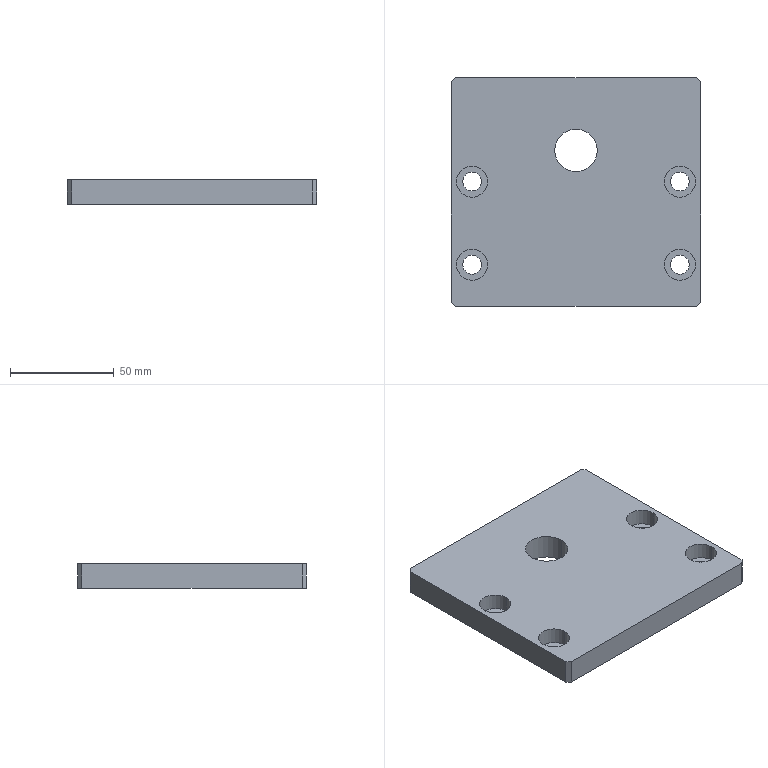Part | SolidWorks | features BaseBody 1 | 1 solid | 32 faces | box 120 x 110 x 12 mm | volume 147670 mm3 | cylinder 18 | plane 14 | commonest cylinder face diameters 9 x8 15 x8 20.5 x2
STEP:
#1=CARTESIAN_POINT('',(54.5,5.,0.));
#2=VERTEX_POINT('',#1);
#3=CARTESIAN_POINT('',(45.5,5.,0.));
#4=VERTEX_POINT('',#3);
#5=CARTESIAN_POINT('',(50.,5.,0.));
#6=DIRECTION('',(0.,0.,-1.));
#7=DIRECTION('',(1.,0.,0.));
#8=AXIS2_PLACEMENT_3D('',#5,#6,#7);
#9=CIRCLE('',#8,4.5);
#10=EDGE_CURVE('',#2,#4,#9,.T.);
#11=ORIENTED_EDGE('',*,*,#10,.T.);
#12=CARTESIAN_POINT('',(45.5,5.,4.));
#13=VERTEX_POINT('',#12);
#14=CARTESIAN_POINT('',(45.5,5.,12.));
#15=DIRECTION('',(0.,0.,1.));
#16=VECTOR('',#15,1000.);
#17=LINE('',#14,#16);
#18=EDGE_CURVE('',#4,#13,#17,.T.);
#19=ORIENTED_EDGE('',*,*,#18,.T.);
#20=CARTESIAN_POINT('',(54.5,5.,4.));
#21=VERTEX_POINT('',#20);
#22=CARTESIAN_POINT('',(50.,5.,4.));
#23=DIRECTION('',(0.,0.,-1.));
#24=DIRECTION('',(1.,0.,0.));
#25=AXIS2_PLACEMENT_3D('',#22,#23,#24);
#26=CIRCLE('',#25,4.5);
#27=EDGE_CURVE('',#21,#13,#26,.T.);
#28=ORIENTED_EDGE('',*,*,#27,.F.);
#29=CARTESIAN_POINT('',(54.5,5.,12.));
#30=DIRECTION('',(0.,0.,1.));
#31=VECTOR('',#30,1000.);
#32=LINE('',#29,#31);
#33=EDGE_CURVE('',#2,#21,#32,.T.);
#34=ORIENTED_EDGE('',*,*,#33,.F.);
#35=EDGE_LOOP('',(#11,#19,#28,#34));
#36=FACE_OUTER_BOUND('',#35,.T.);
#37=CARTESIAN_POINT('',(50.,5.,12.));
#38=DIRECTION('',(0.,0.,1.));
#39=DIRECTION('',(1.,0.,0.));
#40=AXIS2_PLACEMENT_3D('',#37,#38,#39);
#41=CYLINDRICAL_SURFACE('',#40,4.5);
#42=ADVANCED_FACE('',(#36),#41,.F.);
#43=CARTESIAN_POINT('',(54.5,-35.,0.));
#44=VERTEX_POINT('',#43);
#45=CARTESIAN_POINT('',(45.5,-35.,0.));
#46=VERTEX_POINT('',#45);
#47=CARTESIAN_POINT('',(50.,-35.,0.));
#48=DIRECTION('',(0.,0.,-1.));
#49=DIRECTION('',(1.,0.,0.));
#50=AXIS2_PLACEMENT_3D('',#47,#48,#49);
#51=CIRCLE('',#50,4.5);
#52=EDGE_CURVE('',#44,#46,#51,.T.);
#53=ORIENTED_EDGE('',*,*,#52,.T.);
#54=CARTESIAN_POINT('',(45.5,-35.,4.));
#55=VERTEX_POINT('',#54);
#56=CARTESIAN_POINT('',(45.5,-35.,12.));
#57=DIRECTION('',(0.,0.,1.));
#58=VECTOR('',#57,1000.);
#59=LINE('',#56,#58);
#60=EDGE_CURVE('',#46,#55,#59,.T.);
#61=ORIENTED_EDGE('',*,*,#60,.T.);
#62=CARTESIAN_POINT('',(54.5,-35.,4.));
#63=VERTEX_POINT('',#62);
#64=CARTESIAN_POINT('',(50.,-35.,4.));
#65=DIRECTION('',(0.,0.,-1.));
#66=DIRECTION('',(1.,0.,0.));
#67=AXIS2_PLACEMENT_3D('',#64,#65,#66);
#68=CIRCLE('',#67,4.5);
#69=EDGE_CURVE('',#63,#55,#68,.T.);
#70=ORIENTED_EDGE('',*,*,#69,.F.);
#71=CARTESIAN_POINT('',(54.5,-35.,12.));
#72=DIRECTION('',(0.,0.,1.));
#73=VECTOR('',#72,1000.);
#74=LINE('',#71,#73);
#75=EDGE_CURVE('',#44,#63,#74,.T.);
#76=ORIENTED_EDGE('',*,*,#75,.F.);
#77=EDGE_LOOP('',(#53,#61,#70,#76));
#78=FACE_OUTER_BOUND('',#77,.T.);
#79=CARTESIAN_POINT('',(50.,-35.,12.));
#80=DIRECTION('',(0.,0.,1.));
#81=DIRECTION('',(1.,0.,0.));
#82=AXIS2_PLACEMENT_3D('',#79,#80,#81);
#83=CYLINDRICAL_SURFACE('',#82,4.5);
#84=ADVANCED_FACE('',(#78),#83,.F.);
#85=CARTESIAN_POINT('',(-45.5,-35.,0.));
#86=VERTEX_POINT('',#85);
#87=CARTESIAN_POINT('',(-54.5,-35.,0.));
#88=VERTEX_POINT('',#87);
#89=CARTESIAN_POINT('',(-50.,-35.,0.));
#90=DIRECTION('',(0.,0.,-1.));
#91=DIRECTION('',(1.,0.,0.));
#92=AXIS2_PLACEMENT_3D('',#89,#90,#91);
#93=CIRCLE('',#92,4.5);
#94=EDGE_CURVE('',#86,#88,#93,.T.);
#95=ORIENTED_EDGE('',*,*,#94,.T.);
#96=CARTESIAN_POINT('',(-54.5,-35.,4.));
#97=VERTEX_POINT('',#96);
#98=CARTESIAN_POINT('',(-54.5,-35.,12.));
#99=DIRECTION('',(0.,0.,1.));
#100=VECTOR('',#99,1000.);
#101=LINE('',#98,#100);
#102=EDGE_CURVE('',#88,#97,#101,.T.);
#103=ORIENTED_EDGE('',*,*,#102,.T.);
#104=CARTESIAN_POINT('',(-45.5,-35.,4.));
#105=VERTEX_POINT('',#104);
#106=CARTESIAN_POINT('',(-50.,-35.,4.));
#107=DIRECTION('',(0.,0.,-1.));
#108=DIRECTION('',(1.,0.,0.));
#109=AXIS2_PLACEMENT_3D('',#106,#107,#108);
#110=CIRCLE('',#109,4.5);
#111=EDGE_CURVE('',#105,#97,#110,.T.);
#112=ORIENTED_EDGE('',*,*,#111,.F.);
#113=CARTESIAN_POINT('',(-45.5,-35.,12.));
#114=DIRECTION('',(0.,0.,1.));
#115=VECTOR('',#114,1000.);
#116=LINE('',#113,#115);
#117=EDGE_CURVE('',#86,#105,#116,.T.);
#118=ORIENTED_EDGE('',*,*,#117,.F.);
#119=EDGE_LOOP('',(#95,#103,#112,#118));
#120=FACE_OUTER_BOUND('',#119,.T.);
#121=CARTESIAN_POINT('',(-50.,-35.,12.));
#122=DIRECTION('',(0.,0.,1.));
#123=DIRECTION('',(1.,0.,0.));
#124=AXIS2_PLACEMENT_3D('',#121,#122,#123);
#125=CYLINDRICAL_SURFACE('',#124,4.5);
#126=ADVANCED_FACE('',(#120),#125,.F.);
#127=CARTESIAN_POINT('',(-45.5,5.,0.));
#128=VERTEX_POINT('',#127);
#129=CARTESIAN_POINT('',(-54.5,5.,0.));
#130=VERTEX_POINT('',#129);
#131=CARTESIAN_POINT('',(-50.,5.,0.));
#132=DIRECTION('',(0.,0.,-1.));
#133=DIRECTION('',(1.,0.,0.));
#134=AXIS2_PLACEMENT_3D('',#131,#132,#133);
#135=CIRCLE('',#134,4.5);
#136=EDGE_CURVE('',#128,#130,#135,.T.);
#137=ORIENTED_EDGE('',*,*,#136,.T.);
#138=CARTESIAN_POINT('',(-54.5,5.,4.));
#139=VERTEX_POINT('',#138);
#140=CARTESIAN_POINT('',(-54.5,5.,12.));
#141=DIRECTION('',(0.,0.,1.));
#142=VECTOR('',#141,1000.);
#143=LINE('',#140,#142);
#144=EDGE_CURVE('',#130,#139,#143,.T.);
#145=ORIENTED_EDGE('',*,*,#144,.T.);
#146=CARTESIAN_POINT('',(-45.5,5.,4.));
#147=VERTEX_POINT('',#146);
#148=CARTESIAN_POINT('',(-50.,5.,4.));
#149=DIRECTION('',(0.,0.,-1.));
#150=DIRECTION('',(1.,0.,0.));
#151=AXIS2_PLACEMENT_3D('',#148,#149,#150);
#152=CIRCLE('',#151,4.5);
#153=EDGE_CURVE('',#147,#139,#152,.T.);
#154=ORIENTED_EDGE('',*,*,#153,.F.);
#155=CARTESIAN_POINT('',(-45.5,5.,12.));
#156=DIRECTION('',(0.,0.,1.));
#157=VECTOR('',#156,1000.);
#158=LINE('',#155,#157);
#159=EDGE_CURVE('',#128,#147,#158,.T.);
#160=ORIENTED_EDGE('',*,*,#159,.F.);
#161=EDGE_LOOP('',(#137,#145,#154,#160));
#162=FACE_OUTER_BOUND('',#161,.T.);
#163=CARTESIAN_POINT('',(-50.,5.,12.));
#164=DIRECTION('',(0.,0.,1.));
#165=DIRECTION('',(1.,0.,0.));
#166=AXIS2_PLACEMENT_3D('',#163,#164,#165);
#167=CYLINDRICAL_SURFACE('',#166,4.5);
#168=ADVANCED_FACE('',(#162),#167,.F.);
#169=CARTESIAN_POINT('',(10.25,20.,0.));
#170=VERTEX_POINT('',#169);
#171=CARTESIAN_POINT('',(-10.25,20.,0.));
#172=VERTEX_POINT('',#171);
#173=CARTESIAN_POINT('',(0.,20.,0.));
#174=DIRECTION('',(0.,0.,-1.));
#175=DIRECTION('',(1.,0.,0.));
#176=AXIS2_PLACEMENT_3D('',#173,#174,#175);
#177=CIRCLE('',#176,10.25);
#178=EDGE_CURVE('',#170,#172,#177,.T.);
#179=ORIENTED_EDGE('',*,*,#178,.T.);
#180=CARTESIAN_POINT('',(-10.25,20.,12.));
#181=VERTEX_POINT('',#180);
#182=CARTESIAN_POINT('',(-10.25,20.,12.));
#183=DIRECTION('',(0.,0.,1.));
#184=VECTOR('',#183,1000.);
#185=LINE('',#182,#184);
#186=EDGE_CURVE('',#172,#181,#185,.T.);
#187=ORIENTED_EDGE('',*,*,#186,.T.);
#188=CARTESIAN_POINT('',(10.25,20.,12.));
#189=VERTEX_POINT('',#188);
#190=CARTESIAN_POINT('',(0.,20.,12.));
#191=DIRECTION('',(0.,0.,-1.));
#192=DIRECTION('',(1.,0.,0.));
#193=AXIS2_PLACEMENT_3D('',#190,#191,#192);
#194=CIRCLE('',#193,10.25);
#195=EDGE_CURVE('',#189,#181,#194,.T.);
#196=ORIENTED_EDGE('',*,*,#195,.F.);
#197=CARTESIAN_POINT('',(10.25,20.,12.));
#198=DIRECTION('',(0.,0.,1.));
#199=VECTOR('',#198,1000.);
#200=LINE('',#197,#199);
#201=EDGE_CURVE('',#170,#189,#200,.T.);
#202=ORIENTED_EDGE('',*,*,#201,.F.);
#203=EDGE_LOOP('',(#179,#187,#196,#202));
#204=FACE_OUTER_BOUND('',#203,.T.);
#205=CARTESIAN_POINT('',(0.,20.,12.));
#206=DIRECTION('',(0.,0.,1.));
#207=DIRECTION('',(1.,0.,0.));
#208=AXIS2_PLACEMENT_3D('',#205,#206,#207);
#209=CYLINDRICAL_SURFACE('',#208,10.25);
#210=ADVANCED_FACE('',(#204),#209,.F.);
#211=CARTESIAN_POINT('',(57.5,5.,4.));
#212=VERTEX_POINT('',#211);
#213=CARTESIAN_POINT('',(42.5,5.,4.));
#214=VERTEX_POINT('',#213);
#215=CARTESIAN_POINT('',(50.,5.,4.));
#216=DIRECTION('',(0.,0.,-1.));
#217=DIRECTION('',(1.,0.,0.));
#218=AXIS2_PLACEMENT_3D('',#215,#216,#217);
#219=CIRCLE('',#218,7.5);
#220=EDGE_CURVE('',#212,#214,#219,.T.);
#221=ORIENTED_EDGE('',*,*,#220,.T.);
#222=CARTESIAN_POINT('',(42.5,5.,12.));
#223=VERTEX_POINT('',#222);
#224=CARTESIAN_POINT('',(42.5,5.,12.));
#225=DIRECTION('',(0.,0.,1.));
#226=VECTOR('',#225,1000.);
#227=LINE('',#224,#226);
#228=EDGE_CURVE('',#214,#223,#227,.T.);
#229=ORIENTED_EDGE('',*,*,#228,.T.);
#230=CARTESIAN_POINT('',(57.5,5.,12.));
#231=VERTEX_POINT('',#230);
#232=CARTESIAN_POINT('',(50.,5.,12.));
#233=DIRECTION('',(0.,0.,-1.));
#234=DIRECTION('',(1.,0.,0.));
#235=AXIS2_PLACEMENT_3D('',#232,#233,#234);
#236=CIRCLE('',#235,7.5);
#237=EDGE_CURVE('',#231,#223,#236,.T.);
#238=ORIENTED_EDGE('',*,*,#237,.F.);
#239=CARTESIAN_POINT('',(57.5,5.,12.));
#240=DIRECTION('',(0.,0.,1.));
#241=VECTOR('',#240,1000.);
#242=LINE('',#239,#241);
#243=EDGE_CURVE('',#212,#231,#242,.T.);
#244=ORIENTED_EDGE('',*,*,#243,.F.);
#245=EDGE_LOOP('',(#221,#229,#238,#244));
#246=FACE_OUTER_BOUND('',#245,.T.);
#247=CARTESIAN_POINT('',(50.,5.,12.));
#248=DIRECTION('',(0.,0.,1.));
#249=DIRECTION('',(1.,0.,0.));
#250=AXIS2_PLACEMENT_3D('',#247,#248,#249);
#251=CYLINDRICAL_SURFACE('',#250,7.5);
#252=ADVANCED_FACE('',(#246),#251,.F.);
#253=CARTESIAN_POINT('',(57.5,-35.,4.));
#254=VERTEX_POINT('',#253);
#255=CARTESIAN_POINT('',(42.5,-35.,4.));
#256=VERTEX_POINT('',#255);
#257=CARTESIAN_POINT('',(50.,-35.,4.));
#258=DIRECTION('',(0.,0.,-1.));
#259=DIRECTION('',(1.,0.,0.));
#260=AXIS2_PLACEMENT_3D('',#257,#258,#259);
#261=CIRCLE('',#260,7.5);
#262=EDGE_CURVE('',#254,#256,#261,.T.);
#263=ORIENTED_EDGE('',*,*,#262,.T.);
#264=CARTESIAN_POINT('',(42.5,-35.,12.));
#265=VERTEX_POINT('',#264);
#266=CARTESIAN_POINT('',(42.5,-35.,12.));
#267=DIRECTION('',(0.,0.,1.));
#268=VECTOR('',#267,1000.);
#269=LINE('',#266,#268);
#270=EDGE_CURVE('',#256,#265,#269,.T.);
#271=ORIENTED_EDGE('',*,*,#270,.T.);
#272=CARTESIAN_POINT('',(57.5,-35.,12.));
#273=VERTEX_POINT('',#272);
#274=CARTESIAN_POINT('',(50.,-35.,12.));
#275=DIRECTION('',(0.,0.,-1.));
#276=DIRECTION('',(1.,0.,0.));
#277=AXIS2_PLACEMENT_3D('',#274,#275,#276);
#278=CIRCLE('',#277,7.5);
#279=EDGE_CURVE('',#273,#265,#278,.T.);
#280=ORIENTED_EDGE('',*,*,#279,.F.);
#281=CARTESIAN_POINT('',(57.5,-35.,12.));
#282=DIRECTION('',(0.,0.,1.));
#283=VECTOR('',#282,1000.);
#284=LINE('',#281,#283);
#285=EDGE_CURVE('',#254,#273,#284,.T.);
#286=ORIENTED_EDGE('',*,*,#285,.F.);
#287=EDGE_LOOP('',(#263,#271,#280,#286));
#288=FACE_OUTER_BOUND('',#287,.T.);
#289=CARTESIAN_POINT('',(50.,-35.,12.));
#290=DIRECTION('',(0.,0.,1.));
#291=DIRECTION('',(1.,0.,0.));
#292=AXIS2_PLACEMENT_3D('',#289,#290,#291);
#293=CYLINDRICAL_SURFACE('',#292,7.5);
#294=ADVANCED_FACE('',(#288),#293,.F.);
#295=CARTESIAN_POINT('',(-42.5,-35.,4.));
#296=VERTEX_POINT('',#295);
#297=CARTESIAN_POINT('',(-57.5,-35.,4.));
#298=VERTEX_POINT('',#297);
#299=CARTESIAN_POINT('',(-50.,-35.,4.));
#300=DIRECTION('',(0.,0.,-1.));
#301=DIRECTION('',(1.,0.,0.));
#302=AXIS2_PLACEMENT_3D('',#299,#300,#301);
#303=CIRCLE('',#302,7.5);
#304=EDGE_CURVE('',#296,#298,#303,.T.);
#305=ORIENTED_EDGE('',*,*,#304,.T.);
#306=CARTESIAN_POINT('',(-57.5,-35.,12.));
#307=VERTEX_POINT('',#306);
#308=CARTESIAN_POINT('',(-57.5,-35.,12.));
#309=DIRECTION('',(0.,0.,1.));
#310=VECTOR('',#309,1000.);
#311=LINE('',#308,#310);
#312=EDGE_CURVE('',#298,#307,#311,.T.);
#313=ORIENTED_EDGE('',*,*,#312,.T.);
#314=CARTESIAN_POINT('',(-42.5,-35.,12.));
#315=VERTEX_POINT('',#314);
#316=CARTESIAN_POINT('',(-50.,-35.,12.));
#317=DIRECTION('',(0.,0.,-1.));
#318=DIRECTION('',(1.,0.,0.));
#319=AXIS2_PLACEMENT_3D('',#316,#317,#318);
#320=CIRCLE('',#319,7.5);
#321=EDGE_CURVE('',#315,#307,#320,.T.);
#322=ORIENTED_EDGE('',*,*,#321,.F.);
#323=CARTESIAN_POINT('',(-42.5,-35.,12.));
#324=DIRECTION('',(0.,0.,1.));
#325=VECTOR('',#324,1000.);
#326=LINE('',#323,#325);
#327=EDGE_CURVE('',#296,#315,#326,.T.);
#328=ORIENTED_EDGE('',*,*,#327,.F.);
#329=EDGE_LOOP('',(#305,#313,#322,#328));
#330=FACE_OUTER_BOUND('',#329,.T.);
#331=CARTESIAN_POINT('',(-50.,-35.,12.));
#332=DIRECTION('',(0.,0.,1.));
#333=DIRECTION('',(1.,0.,0.));
#334=AXIS2_PLACEMENT_3D('',#331,#332,#333);
#335=CYLINDRICAL_SURFACE('',#334,7.5);
#336=ADVANCED_FACE('',(#330),#335,.F.);
#337=CARTESIAN_POINT('',(-42.5,5.,4.));
#338=VERTEX_POINT('',#337);
#339=CARTESIAN_POINT('',(-57.5,5.,4.));
#340=VERTEX_POINT('',#339);
#341=CARTESIAN_POINT('',(-50.,5.,4.));
#342=DIRECTION('',(0.,0.,-1.));
#343=DIRECTION('',(1.,0.,0.));
#344=AXIS2_PLACEMENT_3D('',#341,#342,#343);
#345=CIRCLE('',#344,7.5);
#346=EDGE_CURVE('',#338,#340,#345,.T.);
#347=ORIENTED_EDGE('',*,*,#346,.T.);
#348=CARTESIAN_POINT('',(-57.5,5.,12.));
#349=VERTEX_POINT('',#348);
#350=CARTESIAN_POINT('',(-57.5,5.,12.));
#351=DIRECTION('',(0.,0.,1.));
#352=VECTOR('',#351,1000.);
#353=LINE('',#350,#352);
#354=EDGE_CURVE('',#340,#349,#353,.T.);
#355=ORIENTED_EDGE('',*,*,#354,.T.);
#356=CARTESIAN_POINT('',(-42.5,5.,12.));
#357=VERTEX_POINT('',#356);
#358=CARTESIAN_POINT('',(-50.,5.,12.));
#359=DIRECTION('',(0.,0.,-1.));
#360=DIRECTION('',(1.,0.,0.));
#361=AXIS2_PLACEMENT_3D('',#358,#359,#360);
#362=CIRCLE('',#361,7.5);
#363=EDGE_CURVE('',#357,#349,#362,.T.);
#364=ORIENTED_EDGE('',*,*,#363,.F.);
#365=CARTESIAN_POINT('',(-42.5,5.,12.));
#366=DIRECTION('',(0.,0.,1.));
#367=VECTOR('',#366,1000.);
#368=LINE('',#365,#367);
#369=EDGE_CURVE('',#338,#357,#368,.T.);
#370=ORIENTED_EDGE('',*,*,#369,.F.);
#371=EDGE_LOOP('',(#347,#355,#364,#370));
#372=FACE_OUTER_BOUND('',#371,.T.);
#373=CARTESIAN_POINT('',(-50.,5.,12.));
#374=DIRECTION('',(0.,0.,1.));
#375=DIRECTION('',(1.,0.,0.));
#376=AXIS2_PLACEMENT_3D('',#373,#374,#375);
#377=CYLINDRICAL_SURFACE('',#376,7.5);
#378=ADVANCED_FACE('',(#372),#377,.F.);
#379=CARTESIAN_POINT('',(-58.,55.,0.));
#380=VERTEX_POINT('',#379);
#381=CARTESIAN_POINT('',(-60.,53.,0.));
#382=VERTEX_POINT('',#381);
#383=CARTESIAN_POINT('',(-58.,55.,0.));
#384=DIRECTION('',(-0.7071,-0.7071,0.));
#385=VECTOR('',#384,1000.);
#386=LINE('',#383,#385);
#387=EDGE_CURVE('',#380,#382,#386,.T.);
#388=ORIENTED_EDGE('',*,*,#387,.F.);
#389=CARTESIAN_POINT('',(58.,55.,0.));
#390=VERTEX_POINT('',#389);
#391=CARTESIAN_POINT('',(0.,55.,0.));
#392=DIRECTION('',(-1.,0.,0.));
#393=VECTOR('',#392,1000.);
#394=LINE('',#391,#393);
#395=EDGE_CURVE('',#390,#380,#394,.T.);
#396=ORIENTED_EDGE('',*,*,#395,.F.);
#397=CARTESIAN_POINT('',(60.,53.,0.));
#398=VERTEX_POINT('',#397);
#399=CARTESIAN_POINT('',(60.,53.,0.));
#400=DIRECTION('',(-0.7071,0.7071,0.));
#401=VECTOR('',#400,1000.);
#402=LINE('',#399,#401);
#403=EDGE_CURVE('',#398,#390,#402,.T.);
#404=ORIENTED_EDGE('',*,*,#403,.F.);
#405=CARTESIAN_POINT('',(60.,-53.,0.));
#406=VERTEX_POINT('',#405);
#407=CARTESIAN_POINT('',(60.,0.,0.));
#408=DIRECTION('',(0.,1.,0.));
#409=VECTOR('',#408,1000.);
#410=LINE('',#407,#409);
#411=EDGE_CURVE('',#406,#398,#410,.T.);
#412=ORIENTED_EDGE('',*,*,#411,.F.);
#413=CARTESIAN_POINT('',(58.,-55.,0.));
#414=VERTEX_POINT('',#413);
#415=CARTESIAN_POINT('',(58.,-55.,0.));
#416=DIRECTION('',(0.7071,0.7071,0.));
#417=VECTOR('',#416,1000.);
#418=LINE('',#415,#417);
#419=EDGE_CURVE('',#414,#406,#418,.T.);
#420=ORIENTED_EDGE('',*,*,#419,.F.);
#421=CARTESIAN_POINT('',(-58.,-55.,0.));
#422=VERTEX_POINT('',#421);
#423=CARTESIAN_POINT('',(0.,-55.,0.));
#424=DIRECTION('',(1.,0.,0.));
#425=VECTOR('',#424,1000.);
#426=LINE('',#423,#425);
#427=EDGE_CURVE('',#422,#414,#426,.T.);
#428=ORIENTED_EDGE('',*,*,#427,.F.);
#429=CARTESIAN_POINT('',(-60.,-53.,0.));
#430=VERTEX_POINT('',#429);
#431=CARTESIAN_POINT('',(-60.,-53.,0.));
#432=DIRECTION('',(0.7071,-0.7071,0.));
#433=VECTOR('',#432,1000.);
#434=LINE('',#431,#433);
#435=EDGE_CURVE('',#430,#422,#434,.T.);
#436=ORIENTED_EDGE('',*,*,#435,.F.);
#437=CARTESIAN_POINT('',(-60.,0.,0.));
#438=DIRECTION('',(0.,-1.,0.));
#439=VECTOR('',#438,1000.);
#440=LINE('',#437,#439);
#441=EDGE_CURVE('',#382,#430,#440,.T.);
#442=ORIENTED_EDGE('',*,*,#441,.F.);
#443=EDGE_LOOP('',(#388,#396,#404,#412,#420,#428,#436,#442));
#444=FACE_OUTER_BOUND('',#443,.T.);
#445=ORIENTED_EDGE('',*,*,#10,.F.);
#446=CARTESIAN_POINT('',(50.,5.,0.));
#447=DIRECTION('',(0.,0.,-1.));
#448=DIRECTION('',(1.,0.,0.));
#449=AXIS2_PLACEMENT_3D('',#446,#447,#448);
#450=CIRCLE('',#449,4.5);
#451=EDGE_CURVE('',#4,#2,#450,.T.);
#452=ORIENTED_EDGE('',*,*,#451,.F.);
#453=EDGE_LOOP('',(#445,#452));
#454=FACE_BOUND('',#453,.T.);
#455=ORIENTED_EDGE('',*,*,#52,.F.);
#456=CARTESIAN_POINT('',(50.,-35.,0.));
#457=DIRECTION('',(0.,0.,-1.));
#458=DIRECTION('',(1.,0.,0.));
#459=AXIS2_PLACEMENT_3D('',#456,#457,#458);
#460=CIRCLE('',#459,4.5);
#461=EDGE_CURVE('',#46,#44,#460,.T.);
#462=ORIENTED_EDGE('',*,*,#461,.F.);
#463=EDGE_LOOP('',(#455,#462));
#464=FACE_BOUND('',#463,.T.);
#465=ORIENTED_EDGE('',*,*,#94,.F.);
#466=CARTESIAN_POINT('',(-50.,-35.,0.));
#467=DIRECTION('',(0.,0.,-1.));
#468=DIRECTION('',(1.,0.,0.));
#469=AXIS2_PLACEMENT_3D('',#466,#467,#468);
#470=CIRCLE('',#469,4.5);
#471=EDGE_CURVE('',#88,#86,#470,.T.);
#472=ORIENTED_EDGE('',*,*,#471,.F.);
#473=EDGE_LOOP('',(#465,#472));
#474=FACE_BOUND('',#473,.T.);
#475=ORIENTED_EDGE('',*,*,#136,.F.);
#476=CARTESIAN_POINT('',(-50.,5.,0.));
#477=DIRECTION('',(0.,0.,-1.));
#478=DIRECTION('',(1.,0.,0.));
#479=AXIS2_PLACEMENT_3D('',#476,#477,#478);
#480=CIRCLE('',#479,4.5);
#481=EDGE_CURVE('',#130,#128,#480,.T.);
#482=ORIENTED_EDGE('',*,*,#481,.F.);
#483=EDGE_LOOP('',(#475,#482));
#484=FACE_BOUND('',#483,.T.);
#485=ORIENTED_EDGE('',*,*,#178,.F.);
#486=CARTESIAN_POINT('',(0.,20.,0.));
#487=DIRECTION('',(0.,0.,-1.));
#488=DIRECTION('',(1.,0.,0.));
#489=AXIS2_PLACEMENT_3D('',#486,#487,#488);
#490=CIRCLE('',#489,10.25);
#491=EDGE_CURVE('',#172,#170,#490,.T.);
#492=ORIENTED_EDGE('',*,*,#491,.F.);
#493=EDGE_LOOP('',(#485,#492));
#494=FACE_BOUND('',#493,.T.);
#495=CARTESIAN_POINT('',(0.,0.,0.));
#496=DIRECTION('',(0.,0.,1.));
#497=DIRECTION('',(1.,0.,0.));
#498=AXIS2_PLACEMENT_3D('',#495,#496,#497);
#499=PLANE('',#498);
#500=ADVANCED_FACE('',(#444,#454,#464,#474,#484,#494),#499,.F.);
#501=CARTESIAN_POINT('',(-60.,53.,12.));
#502=VERTEX_POINT('',#501);
#503=CARTESIAN_POINT('',(-60.,53.,12.));
#504=DIRECTION('',(0.,0.,1.));
#505=VECTOR('',#504,1000.);
#506=LINE('',#503,#505);
#507=EDGE_CURVE('',#382,#502,#506,.T.);
#508=ORIENTED_EDGE('',*,*,#507,.F.);
#509=ORIENTED_EDGE('',*,*,#441,.T.);
#510=CARTESIAN_POINT('',(-60.,-53.,12.));
#511=VERTEX_POINT('',#510);
#512=CARTESIAN_POINT('',(-60.,-53.,12.));
#513=DIRECTION('',(0.,0.,-1.));
#514=VECTOR('',#513,1000.);
#515=LINE('',#512,#514);
#516=EDGE_CURVE('',#511,#430,#515,.T.);
#517=ORIENTED_EDGE('',*,*,#516,.F.);
#518=CARTESIAN_POINT('',(-60.,55.,12.));
#519=DIRECTION('',(0.,-1.,0.));
#520=VECTOR('',#519,1000.);
#521=LINE('',#518,#520);
#522=EDGE_CURVE('',#502,#511,#521,.T.);
#523=ORIENTED_EDGE('',*,*,#522,.F.);
#524=EDGE_LOOP('',(#508,#509,#517,#523));
#525=FACE_OUTER_BOUND('',#524,.T.);
#526=CARTESIAN_POINT('',(-60.,55.,12.));
#527=DIRECTION('',(1.,0.,0.));
#528=DIRECTION('',(0.,1.,0.));
#529=AXIS2_PLACEMENT_3D('',#526,#527,#528);
#530=PLANE('',#529);
#531=ADVANCED_FACE('',(#525),#530,.F.);
#532=CARTESIAN_POINT('',(-58.,55.,12.));
#533=VERTEX_POINT('',#532);
#534=CARTESIAN_POINT('',(-58.,55.,12.));
#535=DIRECTION('',(0.,0.,1.));
#536=VECTOR('',#535,1000.);
#537=LINE('',#534,#536);
#538=EDGE_CURVE('',#380,#533,#537,.T.);
#539=ORIENTED_EDGE('',*,*,#538,.F.);
#540=ORIENTED_EDGE('',*,*,#387,.T.);
#541=ORIENTED_EDGE('',*,*,#507,.T.);
#542=CARTESIAN_POINT('',(-60.,53.,12.));
#543=DIRECTION('',(-0.7071,-0.7071,0.));
#544=VECTOR('',#543,1000.);
#545=LINE('',#542,#544);
#546=EDGE_CURVE('',#533,#502,#545,.T.);
#547=ORIENTED_EDGE('',*,*,#546,.F.);
#548=EDGE_LOOP('',(#539,#540,#541,#547));
#549=FACE_OUTER_BOUND('',#548,.T.);
#550=CARTESIAN_POINT('',(-60.,53.,12.));
#551=DIRECTION('',(0.7071,-0.7071,0.));
#552=DIRECTION('',(0.7071,0.7071,0.));
#553=AXIS2_PLACEMENT_3D('',#550,#551,#552);
#554=PLANE('',#553);
#555=ADVANCED_FACE('',(#549),#554,.F.);
#556=ORIENTED_EDGE('',*,*,#538,.T.);
#557=CARTESIAN_POINT('',(58.,55.,12.));
#558=VERTEX_POINT('',#557);
#559=CARTESIAN_POINT('',(-60.,55.,12.));
#560=DIRECTION('',(-1.,0.,0.));
#561=VECTOR('',#560,1000.);
#562=LINE('',#559,#561);
#563=EDGE_CURVE('',#558,#533,#562,.T.);
#564=ORIENTED_EDGE('',*,*,#563,.F.);
#565=CARTESIAN_POINT('',(58.,55.,12.));
#566=DIRECTION('',(0.,0.,1.));
#567=VECTOR('',#566,1000.);
#568=LINE('',#565,#567);
#569=EDGE_CURVE('',#390,#558,#568,.T.);
#570=ORIENTED_EDGE('',*,*,#569,.F.);
#571=ORIENTED_EDGE('',*,*,#395,.T.);
#572=EDGE_LOOP('',(#556,#564,#570,#571));
#573=FACE_OUTER_BOUND('',#572,.T.);
#574=CARTESIAN_POINT('',(-60.,55.,12.));
#575=DIRECTION('',(0.,-1.,0.));
#576=DIRECTION('',(0.,0.,-1.));
#577=AXIS2_PLACEMENT_3D('',#574,#575,#576);
#578=PLANE('',#577);
#579=ADVANCED_FACE('',(#573),#578,.F.);
#580=CARTESIAN_POINT('',(60.,53.,12.));
#581=VERTEX_POINT('',#580);
#582=CARTESIAN_POINT('',(60.,53.,12.));
#583=DIRECTION('',(0.,0.,1.));
#584=VECTOR('',#583,1000.);
#585=LINE('',#582,#584);
#586=EDGE_CURVE('',#398,#581,#585,.T.);
#587=ORIENTED_EDGE('',*,*,#586,.F.);
#588=ORIENTED_EDGE('',*,*,#403,.T.);
#589=ORIENTED_EDGE('',*,*,#569,.T.);
#590=CARTESIAN_POINT('',(58.,55.,12.));
#591=DIRECTION('',(-0.7071,0.7071,0.));
#592=VECTOR('',#591,1000.);
#593=LINE('',#590,#592);
#594=EDGE_CURVE('',#581,#558,#593,.T.);
#595=ORIENTED_EDGE('',*,*,#594,.F.);
#596=EDGE_LOOP('',(#587,#588,#589,#595));
#597=FACE_OUTER_BOUND('',#596,.T.);
#598=CARTESIAN_POINT('',(58.,55.,12.));
#599=DIRECTION('',(-0.7071,-0.7071,0.));
#600=DIRECTION('',(0.7071,-0.7071,0.));
#601=AXIS2_PLACEMENT_3D('',#598,#599,#600);
#602=PLANE('',#601);
#603=ADVANCED_FACE('',(#597),#602,.F.);
#604=ORIENTED_EDGE('',*,*,#586,.T.);
#605=CARTESIAN_POINT('',(60.,-53.,12.));
#606=VERTEX_POINT('',#605);
#607=CARTESIAN_POINT('',(60.,55.,12.));
#608=DIRECTION('',(0.,1.,0.));
#609=VECTOR('',#608,1000.);
#610=LINE('',#607,#609);
#611=EDGE_CURVE('',#606,#581,#610,.T.);
#612=ORIENTED_EDGE('',*,*,#611,.F.);
#613=CARTESIAN_POINT('',(60.,-53.,12.));
#614=DIRECTION('',(0.,0.,1.));
#615=VECTOR('',#614,1000.);
#616=LINE('',#613,#615);
#617=EDGE_CURVE('',#406,#606,#616,.T.);
#618=ORIENTED_EDGE('',*,*,#617,.F.);
#619=ORIENTED_EDGE('',*,*,#411,.T.);
#620=EDGE_LOOP('',(#604,#612,#618,#619));
#621=FACE_OUTER_BOUND('',#620,.T.);
#622=CARTESIAN_POINT('',(60.,55.,12.));
#623=DIRECTION('',(-1.,0.,0.));
#624=DIRECTION('',(0.,-1.,0.));
#625=AXIS2_PLACEMENT_3D('',#622,#623,#624);
#626=PLANE('',#625);
#627=ADVANCED_FACE('',(#621),#626,.F.);
#628=CARTESIAN_POINT('',(58.,-55.,12.));
#629=VERTEX_POINT('',#628);
#630=CARTESIAN_POINT('',(58.,-55.,12.));
#631=DIRECTION('',(0.,0.,1.));
#632=VECTOR('',#631,1000.);
#633=LINE('',#630,#632);
#634=EDGE_CURVE('',#414,#629,#633,.T.);
#635=ORIENTED_EDGE('',*,*,#634,.F.);
#636=ORIENTED_EDGE('',*,*,#419,.T.);
#637=ORIENTED_EDGE('',*,*,#617,.T.);
#638=CARTESIAN_POINT('',(60.,-53.,12.));
#639=DIRECTION('',(0.7071,0.7071,0.));
#640=VECTOR('',#639,1000.);
#641=LINE('',#638,#640);
#642=EDGE_CURVE('',#629,#606,#641,.T.);
#643=ORIENTED_EDGE('',*,*,#642,.F.);
#644=EDGE_LOOP('',(#635,#636,#637,#643));
#645=FACE_OUTER_BOUND('',#644,.T.);
#646=CARTESIAN_POINT('',(60.,-53.,12.));
#647=DIRECTION('',(-0.7071,0.7071,0.));
#648=DIRECTION('',(-0.7071,-0.7071,0.));
#649=AXIS2_PLACEMENT_3D('',#646,#647,#648);
#650=PLANE('',#649);
#651=ADVANCED_FACE('',(#645),#650,.F.);
#652=ORIENTED_EDGE('',*,*,#634,.T.);
#653=CARTESIAN_POINT('',(-58.,-55.,12.));
#654=VERTEX_POINT('',#653);
#655=CARTESIAN_POINT('',(-60.,-55.,12.));
#656=DIRECTION('',(1.,0.,0.));
#657=VECTOR('',#656,1000.);
#658=LINE('',#655,#657);
#659=EDGE_CURVE('',#654,#629,#658,.T.);
#660=ORIENTED_EDGE('',*,*,#659,.F.);
#661=CARTESIAN_POINT('',(-58.,-55.,12.));
#662=DIRECTION('',(0.,0.,1.));
#663=VECTOR('',#662,1000.);
#664=LINE('',#661,#663);
#665=EDGE_CURVE('',#422,#654,#664,.T.);
#666=ORIENTED_EDGE('',*,*,#665,.F.);
#667=ORIENTED_EDGE('',*,*,#427,.T.);
#668=EDGE_LOOP('',(#652,#660,#666,#667));
#669=FACE_OUTER_BOUND('',#668,.T.);
#670=CARTESIAN_POINT('',(-60.,-55.,12.));
#671=DIRECTION('',(0.,1.,0.));
#672=DIRECTION('',(0.,0.,1.));
#673=AXIS2_PLACEMENT_3D('',#670,#671,#672);
#674=PLANE('',#673);
#675=ADVANCED_FACE('',(#669),#674,.F.);
#676=ORIENTED_EDGE('',*,*,#516,.T.);
#677=ORIENTED_EDGE('',*,*,#435,.T.);
#678=ORIENTED_EDGE('',*,*,#665,.T.);
#679=CARTESIAN_POINT('',(-58.,-55.,12.));
#680=DIRECTION('',(0.7071,-0.7071,0.));
#681=VECTOR('',#680,1000.);
#682=LINE('',#679,#681);
#683=EDGE_CURVE('',#511,#654,#682,.T.);
#684=ORIENTED_EDGE('',*,*,#683,.F.);
#685=EDGE_LOOP('',(#676,#677,#678,#684));
#686=FACE_OUTER_BOUND('',#685,.T.);
#687=CARTESIAN_POINT('',(-58.,-55.,12.));
#688=DIRECTION('',(0.7071,0.7071,0.));
#689=DIRECTION('',(-0.7071,0.7071,0.));
#690=AXIS2_PLACEMENT_3D('',#687,#688,#689);
#691=PLANE('',#690);
#692=ADVANCED_FACE('',(#686),#691,.F.);
#693=ORIENTED_EDGE('',*,*,#18,.F.);
#694=ORIENTED_EDGE('',*,*,#451,.T.);
#695=ORIENTED_EDGE('',*,*,#33,.T.);
#696=CARTESIAN_POINT('',(50.,5.,4.));
#697=DIRECTION('',(0.,0.,-1.));
#698=DIRECTION('',(1.,0.,0.));
#699=AXIS2_PLACEMENT_3D('',#696,#697,#698);
#700=CIRCLE('',#699,4.5);
#701=EDGE_CURVE('',#13,#21,#700,.T.);
#702=ORIENTED_EDGE('',*,*,#701,.F.);
#703=EDGE_LOOP('',(#693,#694,#695,#702));
#704=FACE_OUTER_BOUND('',#703,.T.);
#705=CARTESIAN_POINT('',(50.,5.,12.));
#706=DIRECTION('',(0.,0.,1.));
#707=DIRECTION('',(1.,0.,0.));
#708=AXIS2_PLACEMENT_3D('',#705,#706,#707);
#709=CYLINDRICAL_SURFACE('',#708,4.5);
#710=ADVANCED_FACE('',(#704),#709,.F.);
#711=ORIENTED_EDGE('',*,*,#60,.F.);
#712=ORIENTED_EDGE('',*,*,#461,.T.);
#713=ORIENTED_EDGE('',*,*,#75,.T.);
#714=CARTESIAN_POINT('',(50.,-35.,4.));
#715=DIRECTION('',(0.,0.,-1.));
#716=DIRECTION('',(1.,0.,0.));
#717=AXIS2_PLACEMENT_3D('',#714,#715,#716);
#718=CIRCLE('',#717,4.5);
#719=EDGE_CURVE('',#55,#63,#718,.T.);
#720=ORIENTED_EDGE('',*,*,#719,.F.);
#721=EDGE_LOOP('',(#711,#712,#713,#720));
#722=FACE_OUTER_BOUND('',#721,.T.);
#723=CARTESIAN_POINT('',(50.,-35.,12.));
#724=DIRECTION('',(0.,0.,1.));
#725=DIRECTION('',(1.,0.,0.));
#726=AXIS2_PLACEMENT_3D('',#723,#724,#725);
#727=CYLINDRICAL_SURFACE('',#726,4.5);
#728=ADVANCED_FACE('',(#722),#727,.F.);
#729=ORIENTED_EDGE('',*,*,#102,.F.);
#730=ORIENTED_EDGE('',*,*,#471,.T.);
#731=ORIENTED_EDGE('',*,*,#117,.T.);
#732=CARTESIAN_POINT('',(-50.,-35.,4.));
#733=DIRECTION('',(0.,0.,-1.));
#734=DIRECTION('',(1.,0.,0.));
#735=AXIS2_PLACEMENT_3D('',#732,#733,#734);
#736=CIRCLE('',#735,4.5);
#737=EDGE_CURVE('',#97,#105,#736,.T.);
#738=ORIENTED_EDGE('',*,*,#737,.F.);
#739=EDGE_LOOP('',(#729,#730,#731,#738));
#740=FACE_OUTER_BOUND('',#739,.T.);
#741=CARTESIAN_POINT('',(-50.,-35.,12.));
#742=DIRECTION('',(0.,0.,1.));
#743=DIRECTION('',(1.,0.,0.));
#744=AXIS2_PLACEMENT_3D('',#741,#742,#743);
#745=CYLINDRICAL_SURFACE('',#744,4.5);
#746=ADVANCED_FACE('',(#740),#745,.F.);
#747=ORIENTED_EDGE('',*,*,#144,.F.);
#748=ORIENTED_EDGE('',*,*,#481,.T.);
#749=ORIENTED_EDGE('',*,*,#159,.T.);
#750=CARTESIAN_POINT('',(-50.,5.,4.));
#751=DIRECTION('',(0.,0.,-1.));
#752=DIRECTION('',(1.,0.,0.));
#753=AXIS2_PLACEMENT_3D('',#750,#751,#752);
#754=CIRCLE('',#753,4.5);
#755=EDGE_CURVE('',#139,#147,#754,.T.);
#756=ORIENTED_EDGE('',*,*,#755,.F.);
#757=EDGE_LOOP('',(#747,#748,#749,#756));
#758=FACE_OUTER_BOUND('',#757,.T.);
#759=CARTESIAN_POINT('',(-50.,5.,12.));
#760=DIRECTION('',(0.,0.,1.));
#761=DIRECTION('',(1.,0.,0.));
#762=AXIS2_PLACEMENT_3D('',#759,#760,#761);
#763=CYLINDRICAL_SURFACE('',#762,4.5);
#764=ADVANCED_FACE('',(#758),#763,.F.);
#765=ORIENTED_EDGE('',*,*,#186,.F.);
#766=ORIENTED_EDGE('',*,*,#491,.T.);
#767=ORIENTED_EDGE('',*,*,#201,.T.);
#768=CARTESIAN_POINT('',(0.,20.,12.));
#769=DIRECTION('',(0.,0.,-1.));
#770=DIRECTION('',(1.,0.,0.));
#771=AXIS2_PLACEMENT_3D('',#768,#769,#770);
#772=CIRCLE('',#771,10.25);
#773=EDGE_CURVE('',#181,#189,#772,.T.);
#774=ORIENTED_EDGE('',*,*,#773,.F.);
#775=EDGE_LOOP('',(#765,#766,#767,#774));
#776=FACE_OUTER_BOUND('',#775,.T.);
#777=CARTESIAN_POINT('',(0.,20.,12.));
#778=DIRECTION('',(0.,0.,1.));
#779=DIRECTION('',(1.,0.,0.));
#780=AXIS2_PLACEMENT_3D('',#777,#778,#779);
#781=CYLINDRICAL_SURFACE('',#780,10.25);
#782=ADVANCED_FACE('',(#776),#781,.F.);
#783=ORIENTED_EDGE('',*,*,#611,.T.);
#784=ORIENTED_EDGE('',*,*,#594,.T.);
#785=ORIENTED_EDGE('',*,*,#563,.T.);
#786=ORIENTED_EDGE('',*,*,#546,.T.);
#787=ORIENTED_EDGE('',*,*,#522,.T.);
#788=ORIENTED_EDGE('',*,*,#683,.T.);
#789=ORIENTED_EDGE('',*,*,#659,.T.);
#790=ORIENTED_EDGE('',*,*,#642,.T.);
#791=EDGE_LOOP('',(#783,#784,#785,#786,#787,#788,#789,#790));
#792=FACE_OUTER_BOUND('',#791,.T.);
#793=ORIENTED_EDGE('',*,*,#237,.T.);
#794=CARTESIAN_POINT('',(50.,5.,12.));
#795=DIRECTION('',(0.,0.,-1.));
#796=DIRECTION('',(1.,0.,0.));
#797=AXIS2_PLACEMENT_3D('',#794,#795,#796);
#798=CIRCLE('',#797,7.5);
#799=EDGE_CURVE('',#223,#231,#798,.T.);
#800=ORIENTED_EDGE('',*,*,#799,.T.);
#801=EDGE_LOOP('',(#793,#800));
#802=FACE_BOUND('',#801,.T.);
#803=ORIENTED_EDGE('',*,*,#279,.T.);
#804=CARTESIAN_POINT('',(50.,-35.,12.));
#805=DIRECTION('',(0.,0.,-1.));
#806=DIRECTION('',(1.,0.,0.));
#807=AXIS2_PLACEMENT_3D('',#804,#805,#806);
#808=CIRCLE('',#807,7.5);
#809=EDGE_CURVE('',#265,#273,#808,.T.);
#810=ORIENTED_EDGE('',*,*,#809,.T.);
#811=EDGE_LOOP('',(#803,#810));
#812=FACE_BOUND('',#811,.T.);
#813=ORIENTED_EDGE('',*,*,#321,.T.);
#814=CARTESIAN_POINT('',(-50.,-35.,12.));
#815=DIRECTION('',(0.,0.,-1.));
#816=DIRECTION('',(1.,0.,0.));
#817=AXIS2_PLACEMENT_3D('',#814,#815,#816);
#818=CIRCLE('',#817,7.5);
#819=EDGE_CURVE('',#307,#315,#818,.T.);
#820=ORIENTED_EDGE('',*,*,#819,.T.);
#821=EDGE_LOOP('',(#813,#820));
#822=FACE_BOUND('',#821,.T.);
#823=ORIENTED_EDGE('',*,*,#363,.T.);
#824=CARTESIAN_POINT('',(-50.,5.,12.));
#825=DIRECTION('',(0.,0.,-1.));
#826=DIRECTION('',(1.,0.,0.));
#827=AXIS2_PLACEMENT_3D('',#824,#825,#826);
#828=CIRCLE('',#827,7.5);
#829=EDGE_CURVE('',#349,#357,#828,.T.);
#830=ORIENTED_EDGE('',*,*,#829,.T.);
#831=EDGE_LOOP('',(#823,#830));
#832=FACE_BOUND('',#831,.T.);
#833=ORIENTED_EDGE('',*,*,#195,.T.);
#834=ORIENTED_EDGE('',*,*,#773,.T.);
#835=EDGE_LOOP('',(#833,#834));
#836=FACE_BOUND('',#835,.T.);
#837=CARTESIAN_POINT('',(0.,0.,12.));
#838=DIRECTION('',(0.,0.,1.));
#839=DIRECTION('',(1.,0.,0.));
#840=AXIS2_PLACEMENT_3D('',#837,#838,#839);
#841=PLANE('',#840);
#842=ADVANCED_FACE('',(#792,#802,#812,#822,#832,#836),#841,.T.);
#843=ORIENTED_EDGE('',*,*,#220,.F.);
#844=CARTESIAN_POINT('',(50.,5.,4.));
#845=DIRECTION('',(0.,0.,-1.));
#846=DIRECTION('',(1.,0.,0.));
#847=AXIS2_PLACEMENT_3D('',#844,#845,#846);
#848=CIRCLE('',#847,7.5);
#849=EDGE_CURVE('',#214,#212,#848,.T.);
#850=ORIENTED_EDGE('',*,*,#849,.F.);
#851=EDGE_LOOP('',(#843,#850));
#852=FACE_OUTER_BOUND('',#851,.T.);
#853=ORIENTED_EDGE('',*,*,#27,.T.);
#854=ORIENTED_EDGE('',*,*,#701,.T.);
#855=EDGE_LOOP('',(#853,#854));
#856=FACE_BOUND('',#855,.T.);
#857=CARTESIAN_POINT('',(54.5,5.,4.));
#858=DIRECTION('',(0.,0.,-1.));
#859=DIRECTION('',(-1.,0.,0.));
#860=AXIS2_PLACEMENT_3D('',#857,#858,#859);
#861=PLANE('',#860);
#862=ADVANCED_FACE('',(#852,#856),#861,.F.);
#863=ORIENTED_EDGE('',*,*,#262,.F.);
#864=CARTESIAN_POINT('',(50.,-35.,4.));
#865=DIRECTION('',(0.,0.,-1.));
#866=DIRECTION('',(1.,0.,0.));
#867=AXIS2_PLACEMENT_3D('',#864,#865,#866);
#868=CIRCLE('',#867,7.5);
#869=EDGE_CURVE('',#256,#254,#868,.T.);
#870=ORIENTED_EDGE('',*,*,#869,.F.);
#871=EDGE_LOOP('',(#863,#870));
#872=FACE_OUTER_BOUND('',#871,.T.);
#873=ORIENTED_EDGE('',*,*,#69,.T.);
#874=ORIENTED_EDGE('',*,*,#719,.T.);
#875=EDGE_LOOP('',(#873,#874));
#876=FACE_BOUND('',#875,.T.);
#877=CARTESIAN_POINT('',(54.5,-35.,4.));
#878=DIRECTION('',(0.,0.,-1.));
#879=DIRECTION('',(-1.,0.,0.));
#880=AXIS2_PLACEMENT_3D('',#877,#878,#879);
#881=PLANE('',#880);
#882=ADVANCED_FACE('',(#872,#876),#881,.F.);
#883=ORIENTED_EDGE('',*,*,#304,.F.);
#884=CARTESIAN_POINT('',(-50.,-35.,4.));
#885=DIRECTION('',(0.,0.,-1.));
#886=DIRECTION('',(1.,0.,0.));
#887=AXIS2_PLACEMENT_3D('',#884,#885,#886);
#888=CIRCLE('',#887,7.5);
#889=EDGE_CURVE('',#298,#296,#888,.T.);
#890=ORIENTED_EDGE('',*,*,#889,.F.);
#891=EDGE_LOOP('',(#883,#890));
#892=FACE_OUTER_BOUND('',#891,.T.);
#893=ORIENTED_EDGE('',*,*,#111,.T.);
#894=ORIENTED_EDGE('',*,*,#737,.T.);
#895=EDGE_LOOP('',(#893,#894));
#896=FACE_BOUND('',#895,.T.);
#897=CARTESIAN_POINT('',(-45.5,-35.,4.));
#898=DIRECTION('',(0.,0.,-1.));
#899=DIRECTION('',(-1.,0.,0.));
#900=AXIS2_PLACEMENT_3D('',#897,#898,#899);
#901=PLANE('',#900);
#902=ADVANCED_FACE('',(#892,#896),#901,.F.);
#903=ORIENTED_EDGE('',*,*,#346,.F.);
#904=CARTESIAN_POINT('',(-50.,5.,4.));
#905=DIRECTION('',(0.,0.,-1.));
#906=DIRECTION('',(1.,0.,0.));
#907=AXIS2_PLACEMENT_3D('',#904,#905,#906);
#908=CIRCLE('',#907,7.5);
#909=EDGE_CURVE('',#340,#338,#908,.T.);
#910=ORIENTED_EDGE('',*,*,#909,.F.);
#911=EDGE_LOOP('',(#903,#910));
#912=FACE_OUTER_BOUND('',#911,.T.);
#913=ORIENTED_EDGE('',*,*,#153,.T.);
#914=ORIENTED_EDGE('',*,*,#755,.T.);
#915=EDGE_LOOP('',(#913,#914));
#916=FACE_BOUND('',#915,.T.);
#917=CARTESIAN_POINT('',(-45.5,5.,4.));
#918=DIRECTION('',(0.,0.,-1.));
#919=DIRECTION('',(-1.,0.,0.));
#920=AXIS2_PLACEMENT_3D('',#917,#918,#919);
#921=PLANE('',#920);
#922=ADVANCED_FACE('',(#912,#916),#921,.F.);
#923=ORIENTED_EDGE('',*,*,#228,.F.);
#924=ORIENTED_EDGE('',*,*,#849,.T.);
#925=ORIENTED_EDGE('',*,*,#243,.T.);
#926=ORIENTED_EDGE('',*,*,#799,.F.);
#927=EDGE_LOOP('',(#923,#924,#925,#926));
#928=FACE_OUTER_BOUND('',#927,.T.);
#929=CARTESIAN_POINT('',(50.,5.,12.));
#930=DIRECTION('',(0.,0.,1.));
#931=DIRECTION('',(1.,0.,0.));
#932=AXIS2_PLACEMENT_3D('',#929,#930,#931);
#933=CYLINDRICAL_SURFACE('',#932,7.5);
#934=ADVANCED_FACE('',(#928),#933,.F.);
#935=ORIENTED_EDGE('',*,*,#270,.F.);
#936=ORIENTED_EDGE('',*,*,#869,.T.);
#937=ORIENTED_EDGE('',*,*,#285,.T.);
#938=ORIENTED_EDGE('',*,*,#809,.F.);
#939=EDGE_LOOP('',(#935,#936,#937,#938));
#940=FACE_OUTER_BOUND('',#939,.T.);
#941=CARTESIAN_POINT('',(50.,-35.,12.));
#942=DIRECTION('',(0.,0.,1.));
#943=DIRECTION('',(1.,0.,0.));
#944=AXIS2_PLACEMENT_3D('',#941,#942,#943);
#945=CYLINDRICAL_SURFACE('',#944,7.5);
#946=ADVANCED_FACE('',(#940),#945,.F.);
#947=ORIENTED_EDGE('',*,*,#312,.F.);
#948=ORIENTED_EDGE('',*,*,#889,.T.);
#949=ORIENTED_EDGE('',*,*,#327,.T.);
#950=ORIENTED_EDGE('',*,*,#819,.F.);
#951=EDGE_LOOP('',(#947,#948,#949,#950));
#952=FACE_OUTER_BOUND('',#951,.T.);
#953=CARTESIAN_POINT('',(-50.,-35.,12.));
#954=DIRECTION('',(0.,0.,1.));
#955=DIRECTION('',(1.,0.,0.));
#956=AXIS2_PLACEMENT_3D('',#953,#954,#955);
#957=CYLINDRICAL_SURFACE('',#956,7.5);
#958=ADVANCED_FACE('',(#952),#957,.F.);
#959=ORIENTED_EDGE('',*,*,#354,.F.);
#960=ORIENTED_EDGE('',*,*,#909,.T.);
#961=ORIENTED_EDGE('',*,*,#369,.T.);
#962=ORIENTED_EDGE('',*,*,#829,.F.);
#963=EDGE_LOOP('',(#959,#960,#961,#962));
#964=FACE_OUTER_BOUND('',#963,.T.);
#965=CARTESIAN_POINT('',(-50.,5.,12.));
#966=DIRECTION('',(0.,0.,1.));
#967=DIRECTION('',(1.,0.,0.));
#968=AXIS2_PLACEMENT_3D('',#965,#966,#967);
#969=CYLINDRICAL_SURFACE('',#968,7.5);
#970=ADVANCED_FACE('',(#964),#969,.F.);
#971=CLOSED_SHELL('',(#42,#84,#126,#168,#210,#252,#294,#336,#378,#500,#531,#555,#579,#603,#627,#651,#675,#692,#710,#728,#746,#764,#782,#842,#862,#882,#902,#922,#934,#946,#958,#970));
#972=MANIFOLD_SOLID_BREP('',#971);
#973=CARTESIAN_POINT('',(0.,0.,0.));
#974=DIRECTION('',(0.,0.,1.));
#975=DIRECTION('',(1.,0.,0.));
#976=AXIS2_PLACEMENT_3D('',#973,#974,#975);
#977=(LENGTH_UNIT()NAMED_UNIT(*)SI_UNIT(.MILLI.,.METRE.));
#978=UNCERTAINTY_MEASURE_WITH_UNIT(LENGTH_MEASURE(0.00001),#977,'','');
#979=(NAMED_UNIT(*)PLANE_ANGLE_UNIT()SI_UNIT($,.RADIAN.));
#980=(NAMED_UNIT(*)SI_UNIT($,.STERADIAN.)SOLID_ANGLE_UNIT());
#981=(GEOMETRIC_REPRESENTATION_CONTEXT(3)GLOBAL_UNCERTAINTY_ASSIGNED_CONTEXT((#978))GLOBAL_UNIT_ASSIGNED_CONTEXT((#977,#979,#980))REPRESENTATION_CONTEXT('',''));
#982=ADVANCED_BREP_SHAPE_REPRESENTATION('',(#972,#976),#981);